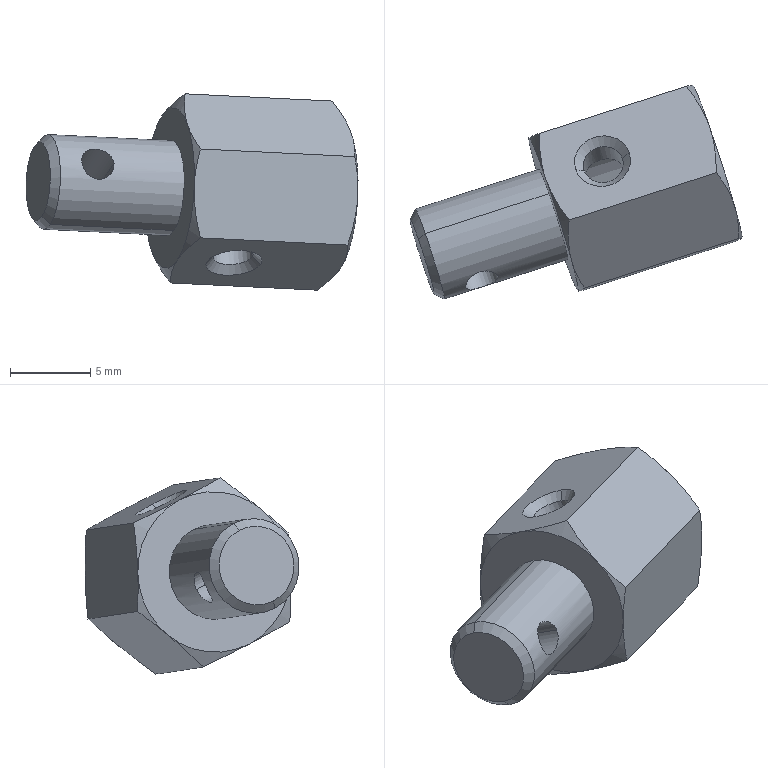Part | SolidWorks | features BaseBody 1 | 1 solid | 41 faces | box 20.658 x 13.325 x 12.212 mm | volume 845.345 mm3 | cone 22 | cylinder 10 | plane 9 | commonest cylinder face diameters 2.5 x4 2.1 x2 5.9 x2 6 x2
STEP:
#1=CARTESIAN_POINT('',(61.625,-75.237,-185.721));
#2=VERTEX_POINT('',#1);
#3=CARTESIAN_POINT('',(63.623,-74.596,-185.819));
#4=VERTEX_POINT('',#3);
#5=CARTESIAN_POINT('',(61.625,-75.237,-185.721));
#6=CARTESIAN_POINT('',(61.639,-75.298,-185.847));
#7=CARTESIAN_POINT('',(61.681,-75.358,-185.966));
#8=CARTESIAN_POINT('',(61.817,-75.465,-186.183));
#9=CARTESIAN_POINT('',(61.908,-75.512,-186.279));
#10=CARTESIAN_POINT('',(62.125,-75.58,-186.439));
#11=CARTESIAN_POINT('',(62.25,-75.6,-186.502));
#12=CARTESIAN_POINT('',(62.511,-75.599,-186.592));
#13=CARTESIAN_POINT('',(62.649,-75.578,-186.619));
#14=CARTESIAN_POINT('',(62.912,-75.494,-186.632));
#15=CARTESIAN_POINT('',(63.038,-75.43,-186.619));
#16=CARTESIAN_POINT('',(63.259,-75.275,-186.552));
#17=CARTESIAN_POINT('',(63.353,-75.186,-186.499));
#18=CARTESIAN_POINT('',(63.504,-75.,-186.357));
#19=CARTESIAN_POINT('',(63.559,-74.905,-186.268));
#20=CARTESIAN_POINT('',(63.625,-74.733,-186.061));
#21=CARTESIAN_POINT('',(63.636,-74.656,-185.943));
#22=CARTESIAN_POINT('',(63.623,-74.596,-185.819));
#23=B_SPLINE_CURVE_WITH_KNOTS('',3,(#5,#6,#7,#8,#9,#10,#11,#12,#13,#14,#15,#16,#17,#18,#19,#20,#21,#22),.UNSPECIFIED.,.F.,.F.,(4,2,2,2,2,2,2,2,4),(0.,0.000413,0.0008261,0.001239,0.001652,0.002065,0.002478,0.002891,0.003304),.UNSPECIFIED.);
#24=EDGE_CURVE('',#2,#4,#23,.T.);
#25=ORIENTED_EDGE('',*,*,#24,.T.);
#26=CARTESIAN_POINT('',(63.623,-74.596,-185.819));
#27=CARTESIAN_POINT('',(63.609,-74.536,-185.696));
#28=CARTESIAN_POINT('',(63.572,-74.493,-185.565));
#29=CARTESIAN_POINT('',(63.459,-74.445,-185.318));
#30=CARTESIAN_POINT('',(63.381,-74.439,-185.2));
#31=CARTESIAN_POINT('',(63.194,-74.457,-184.996));
#32=CARTESIAN_POINT('',(63.085,-74.48,-184.91));
#33=CARTESIAN_POINT('',(62.842,-74.543,-184.786));
#34=CARTESIAN_POINT('',(62.711,-74.583,-184.75));
#35=CARTESIAN_POINT('',(62.448,-74.667,-184.738));
#36=CARTESIAN_POINT('',(62.316,-74.713,-184.761));
#37=CARTESIAN_POINT('',(62.075,-74.804,-184.86));
#38=CARTESIAN_POINT('',(61.965,-74.852,-184.936));
#39=CARTESIAN_POINT('',(61.786,-74.952,-185.121));
#40=CARTESIAN_POINT('',(61.715,-75.005,-185.232));
#41=CARTESIAN_POINT('',(61.628,-75.117,-185.47));
#42=CARTESIAN_POINT('',(61.612,-75.177,-185.596));
#43=CARTESIAN_POINT('',(61.625,-75.237,-185.721));
#44=B_SPLINE_CURVE_WITH_KNOTS('',3,(#26,#27,#28,#29,#30,#31,#32,#33,#34,#35,#36,#37,#38,#39,#40,#41,#42,#43),.UNSPECIFIED.,.F.,.F.,(4,2,2,2,2,2,2,2,4),(0.003304,0.003717,0.004131,0.004544,0.004957,0.00537,0.005783,0.006196,0.006609),.UNSPECIFIED.);
#45=EDGE_CURVE('',#4,#2,#44,.T.);
#46=ORIENTED_EDGE('',*,*,#45,.T.);
#47=EDGE_LOOP('',(#25,#46));
#48=FACE_BOUND('',#47,.T.);
#49=CARTESIAN_POINT('',(61.395,-79.461,-186.994));
#50=VERTEX_POINT('',#49);
#51=CARTESIAN_POINT('',(60.832,-76.901,-181.708));
#52=VERTEX_POINT('',#51);
#53=CARTESIAN_POINT('',(61.113,-78.181,-184.351));
#54=DIRECTION('',(0.9511,0.3055,-0.04654));
#55=DIRECTION('',(-0.09549,0.4338,0.8959));
#56=AXIS2_PLACEMENT_3D('',#53,#54,#55);
#57=CIRCLE('',#56,2.95);
#58=EDGE_CURVE('',#50,#52,#57,.T.);
#59=ORIENTED_EDGE('',*,*,#58,.T.);
#60=CARTESIAN_POINT('',(68.535,-74.427,-182.085));
#61=VERTEX_POINT('',#60);
#62=CARTESIAN_POINT('',(60.356,-77.054,-181.684));
#63=DIRECTION('',(0.9511,0.3055,-0.04654));
#64=VECTOR('',#63,1000.);
#65=LINE('',#62,#64);
#66=EDGE_CURVE('',#52,#61,#65,.T.);
#67=ORIENTED_EDGE('',*,*,#66,.T.);
#68=CARTESIAN_POINT('',(69.099,-76.986,-187.371));
#69=VERTEX_POINT('',#68);
#70=CARTESIAN_POINT('',(68.817,-75.707,-184.728));
#71=DIRECTION('',(-0.9511,-0.3055,0.04654));
#72=DIRECTION('',(0.09549,-0.4338,-0.8959));
#73=AXIS2_PLACEMENT_3D('',#70,#71,#72);
#74=CIRCLE('',#73,2.95);
#75=EDGE_CURVE('',#61,#69,#74,.T.);
#76=ORIENTED_EDGE('',*,*,#75,.T.);
#77=CARTESIAN_POINT('',(60.919,-79.613,-186.971));
#78=DIRECTION('',(0.9511,0.3055,-0.04654));
#79=VECTOR('',#78,1000.);
#80=LINE('',#77,#79);
#81=EDGE_CURVE('',#50,#69,#80,.T.);
#82=ORIENTED_EDGE('',*,*,#81,.F.);
#83=EDGE_LOOP('',(#59,#67,#76,#82));
#84=FACE_OUTER_BOUND('',#83,.T.);
#85=CARTESIAN_POINT('',(60.638,-78.334,-184.328));
#86=DIRECTION('',(0.9511,0.3055,-0.04654));
#87=DIRECTION('',(0.09549,-0.4338,-0.8959));
#88=AXIS2_PLACEMENT_3D('',#85,#86,#87);
#89=CYLINDRICAL_SURFACE('',#88,2.95);
#90=ADVANCED_FACE('',(#48,#84),#89,.T.);
#91=CARTESIAN_POINT('',(60.404,-77.271,-182.132));
#92=VERTEX_POINT('',#91);
#93=CARTESIAN_POINT('',(60.872,-79.396,-186.523));
#94=VERTEX_POINT('',#93);
#95=CARTESIAN_POINT('',(60.638,-78.334,-184.328));
#96=DIRECTION('',(-0.9511,-0.3055,0.04654));
#97=DIRECTION('',(-0.09549,0.4338,0.8959));
#98=AXIS2_PLACEMENT_3D('',#95,#96,#97);
#99=CIRCLE('',#98,2.45);
#100=EDGE_CURVE('',#92,#94,#99,.T.);
#101=ORIENTED_EDGE('',*,*,#100,.F.);
#102=CARTESIAN_POINT('',(60.404,-77.271,-182.132));
#103=DIRECTION('',(0.605,0.5227,0.6006));
#104=VECTOR('',#103,1000.);
#105=LINE('',#102,#104);
#106=EDGE_CURVE('',#92,#52,#105,.T.);
#107=ORIENTED_EDGE('',*,*,#106,.T.);
#108=ORIENTED_EDGE('',*,*,#58,.F.);
#109=CARTESIAN_POINT('',(60.872,-79.396,-186.523));
#110=DIRECTION('',(0.74,-0.09071,-0.6664));
#111=VECTOR('',#110,1000.);
#112=LINE('',#109,#111);
#113=EDGE_CURVE('',#94,#50,#112,.T.);
#114=ORIENTED_EDGE('',*,*,#113,.F.);
#115=EDGE_LOOP('',(#101,#107,#108,#114));
#116=FACE_OUTER_BOUND('',#115,.T.);
#117=CARTESIAN_POINT('',(60.638,-78.334,-184.328));
#118=DIRECTION('',(0.9511,0.3055,-0.04654));
#119=DIRECTION('',(0.09549,-0.4338,-0.8959));
#120=AXIS2_PLACEMENT_3D('',#117,#118,#119);
#121=CONICAL_SURFACE('',#120,2.45,0.7854);
#122=ADVANCED_FACE('',(#116),#121,.T.);
#123=CARTESIAN_POINT('',(70.147,-73.886,-182.119));
#124=VERTEX_POINT('',#123);
#125=CARTESIAN_POINT('',(70.72,-76.488,-187.495));
#126=VERTEX_POINT('',#125);
#127=CARTESIAN_POINT('',(70.434,-75.187,-184.807));
#128=DIRECTION('',(0.9511,0.3055,-0.04654));
#129=DIRECTION('',(0.09549,-0.4338,-0.8959));
#130=AXIS2_PLACEMENT_3D('',#127,#128,#129);
#131=CIRCLE('',#130,3.);
#132=EDGE_CURVE('',#124,#126,#131,.T.);
#133=ORIENTED_EDGE('',*,*,#132,.F.);
#134=CARTESIAN_POINT('',(70.86,-73.657,-182.154));
#135=VERTEX_POINT('',#134);
#136=CARTESIAN_POINT('',(70.147,-73.886,-182.119));
#137=DIRECTION('',(0.9511,0.3055,-0.04654));
#138=VECTOR('',#137,1000.);
#139=LINE('',#136,#138);
#140=EDGE_CURVE('',#124,#135,#139,.T.);
#141=ORIENTED_EDGE('',*,*,#140,.T.);
#142=CARTESIAN_POINT('',(73.238,-72.893,-182.27));
#143=VERTEX_POINT('',#142);
#144=CARTESIAN_POINT('',(70.86,-73.657,-182.154));
#145=CARTESIAN_POINT('',(70.909,-73.796,-182.081));
#146=CARTESIAN_POINT('',(70.991,-73.933,-182.022));
#147=CARTESIAN_POINT('',(71.204,-74.172,-181.939));
#148=CARTESIAN_POINT('',(71.335,-74.275,-181.913));
#149=CARTESIAN_POINT('',(71.555,-74.391,-181.893));
#150=CARTESIAN_POINT('',(71.631,-74.423,-181.889));
#151=CARTESIAN_POINT('',(71.788,-74.473,-181.885));
#152=CARTESIAN_POINT('',(71.871,-74.491,-181.885));
#153=CARTESIAN_POINT('',(72.035,-74.509,-181.888));
#154=CARTESIAN_POINT('',(72.117,-74.51,-181.891));
#155=CARTESIAN_POINT('',(72.281,-74.495,-181.897));
#156=CARTESIAN_POINT('',(72.364,-74.478,-181.901));
#157=CARTESIAN_POINT('',(72.599,-74.403,-181.912));
#158=CARTESIAN_POINT('',(72.746,-74.317,-181.92));
#159=CARTESIAN_POINT('',(72.99,-74.095,-181.943));
#160=CARTESIAN_POINT('',(73.09,-73.96,-181.958));
#161=CARTESIAN_POINT('',(73.234,-73.665,-182.006));
#162=CARTESIAN_POINT('',(73.278,-73.507,-182.04));
#163=CARTESIAN_POINT('',(73.305,-73.189,-182.136));
#164=CARTESIAN_POINT('',(73.287,-73.035,-182.196));
#165=CARTESIAN_POINT('',(73.238,-72.893,-182.27));
#166=B_SPLINE_CURVE_WITH_KNOTS('',3,(#144,#145,#146,#147,#148,#149,#150,#151,#152,#153,#154,#155,#156,#157,#158,#159,#160,#161,#162,#163,#164,#165),.UNSPECIFIED.,.F.,.F.,(4,2,2,2,2,2,2,2,2,2,4),(0.003954,0.004448,0.004941,0.005188,0.005435,0.005682,0.005929,0.006423,0.006917,0.00741,0.007904),.UNSPECIFIED.);
#167=EDGE_CURVE('',#135,#143,#166,.T.);
#168=ORIENTED_EDGE('',*,*,#167,.T.);
#169=CARTESIAN_POINT('',(78.231,-71.289,-182.515));
#170=VERTEX_POINT('',#169);
#171=CARTESIAN_POINT('',(70.147,-73.886,-182.119));
#172=DIRECTION('',(0.9511,0.3055,-0.04654));
#173=VECTOR('',#172,1000.);
#174=LINE('',#171,#173);
#175=EDGE_CURVE('',#143,#170,#174,.T.);
#176=ORIENTED_EDGE('',*,*,#175,.T.);
#177=CARTESIAN_POINT('',(78.804,-73.892,-187.89));
#178=VERTEX_POINT('',#177);
#179=CARTESIAN_POINT('',(78.518,-72.59,-185.202));
#180=DIRECTION('',(0.9511,0.3055,-0.04654));
#181=DIRECTION('',(0.09549,-0.4338,-0.8959));
#182=AXIS2_PLACEMENT_3D('',#179,#180,#181);
#183=CIRCLE('',#182,3.);
#184=EDGE_CURVE('',#170,#178,#183,.T.);
#185=ORIENTED_EDGE('',*,*,#184,.T.);
#186=CARTESIAN_POINT('',(73.811,-75.496,-187.646));
#187=VERTEX_POINT('',#186);
#188=CARTESIAN_POINT('',(70.72,-76.488,-187.495));
#189=DIRECTION('',(0.9511,0.3055,-0.04654));
#190=VECTOR('',#189,1000.);
#191=LINE('',#188,#190);
#192=EDGE_CURVE('',#187,#178,#191,.T.);
#193=ORIENTED_EDGE('',*,*,#192,.F.);
#194=CARTESIAN_POINT('',(71.433,-76.259,-187.53));
#195=VERTEX_POINT('',#194);
#196=CARTESIAN_POINT('',(73.811,-75.496,-187.646));
#197=CARTESIAN_POINT('',(73.859,-75.635,-187.573));
#198=CARTESIAN_POINT('',(73.875,-75.78,-187.486));
#199=CARTESIAN_POINT('',(73.839,-76.054,-187.302));
#200=CARTESIAN_POINT('',(73.788,-76.183,-187.206));
#201=CARTESIAN_POINT('',(73.67,-76.358,-187.075));
#202=CARTESIAN_POINT('',(73.624,-76.413,-187.033));
#203=CARTESIAN_POINT('',(73.52,-76.516,-186.958));
#204=CARTESIAN_POINT('',(73.46,-76.564,-186.923));
#205=CARTESIAN_POINT('',(73.333,-76.652,-186.865));
#206=CARTESIAN_POINT('',(73.265,-76.692,-186.841));
#207=CARTESIAN_POINT('',(73.12,-76.762,-186.806));
#208=CARTESIAN_POINT('',(73.042,-76.793,-186.795));
#209=CARTESIAN_POINT('',(72.807,-76.869,-186.784));
#210=CARTESIAN_POINT('',(72.641,-76.898,-186.805));
#211=CARTESIAN_POINT('',(72.323,-76.906,-186.893));
#212=CARTESIAN_POINT('',(72.169,-76.886,-186.96));
#213=CARTESIAN_POINT('',(71.89,-76.792,-187.114));
#214=CARTESIAN_POINT('',(71.766,-76.72,-187.2));
#215=CARTESIAN_POINT('',(71.56,-76.523,-187.373));
#216=CARTESIAN_POINT('',(71.482,-76.401,-187.456));
#217=CARTESIAN_POINT('',(71.433,-76.259,-187.53));
#218=B_SPLINE_CURVE_WITH_KNOTS('',3,(#196,#197,#198,#199,#200,#201,#202,#203,#204,#205,#206,#207,#208,#209,#210,#211,#212,#213,#214,#215,#216,#217),.UNSPECIFIED.,.F.,.F.,(4,2,2,2,2,2,2,2,2,2,4),(0.003954,0.004448,0.004941,0.005188,0.005435,0.005682,0.005929,0.006423,0.006917,0.00741,0.007904),.UNSPECIFIED.);
#219=EDGE_CURVE('',#187,#195,#218,.T.);
#220=ORIENTED_EDGE('',*,*,#219,.T.);
#221=CARTESIAN_POINT('',(70.72,-76.488,-187.495));
#222=DIRECTION('',(0.9511,0.3055,-0.04654));
#223=VECTOR('',#222,1000.);
#224=LINE('',#221,#223);
#225=EDGE_CURVE('',#126,#195,#224,.T.);
#226=ORIENTED_EDGE('',*,*,#225,.F.);
#227=EDGE_LOOP('',(#133,#141,#168,#176,#185,#193,#220,#226));
#228=FACE_OUTER_BOUND('',#227,.T.);
#229=CARTESIAN_POINT('',(70.434,-75.187,-184.807));
#230=DIRECTION('',(0.9511,0.3055,-0.04654));
#231=DIRECTION('',(0.09549,-0.4338,-0.8959));
#232=AXIS2_PLACEMENT_3D('',#229,#230,#231);
#233=CYLINDRICAL_SURFACE('',#232,3.);
#234=ADVANCED_FACE('',(#228),#233,.F.);
#235=CARTESIAN_POINT('',(68.786,-75.716,-184.726));
#236=VERTEX_POINT('',#235);
#237=CARTESIAN_POINT('',(70.72,-76.488,-187.495));
#238=DIRECTION('',(0.5582,-0.2229,-0.7992));
#239=VECTOR('',#238,1000.);
#240=LINE('',#237,#239);
#241=EDGE_CURVE('',#236,#126,#240,.T.);
#242=ORIENTED_EDGE('',*,*,#241,.F.);
#243=CARTESIAN_POINT('',(70.147,-73.886,-182.119));
#244=DIRECTION('',(0.3928,0.5284,0.7526));
#245=VECTOR('',#244,1000.);
#246=LINE('',#243,#245);
#247=EDGE_CURVE('',#236,#124,#246,.T.);
#248=ORIENTED_EDGE('',*,*,#247,.T.);
#249=ORIENTED_EDGE('',*,*,#132,.T.);
#250=EDGE_LOOP('',(#242,#248,#249));
#251=FACE_OUTER_BOUND('',#250,.T.);
#252=CARTESIAN_POINT('',(70.434,-75.187,-184.807));
#253=DIRECTION('',(0.9511,0.3055,-0.04654));
#254=DIRECTION('',(0.09549,-0.4338,-0.8959));
#255=AXIS2_PLACEMENT_3D('',#252,#253,#254);
#256=CONICAL_SURFACE('',#255,3.,1.047);
#257=ADVANCED_FACE('',(#251),#256,.F.);
#258=ORIENTED_EDGE('',*,*,#184,.F.);
#259=CARTESIAN_POINT('',(78.659,-70.92,-182.09));
#260=VERTEX_POINT('',#259);
#261=CARTESIAN_POINT('',(78.231,-71.289,-182.515));
#262=DIRECTION('',(0.605,0.5227,0.6006));
#263=VECTOR('',#262,1000.);
#264=LINE('',#261,#263);
#265=EDGE_CURVE('',#170,#260,#264,.T.);
#266=ORIENTED_EDGE('',*,*,#265,.T.);
#267=CARTESIAN_POINT('',(79.327,-73.956,-188.362));
#268=VERTEX_POINT('',#267);
#269=CARTESIAN_POINT('',(78.993,-72.438,-185.226));
#270=DIRECTION('',(-0.9511,-0.3055,0.04654));
#271=DIRECTION('',(0.09549,-0.4338,-0.8959));
#272=AXIS2_PLACEMENT_3D('',#269,#270,#271);
#273=CIRCLE('',#272,3.5);
#274=EDGE_CURVE('',#268,#260,#273,.T.);
#275=ORIENTED_EDGE('',*,*,#274,.F.);
#276=CARTESIAN_POINT('',(78.804,-73.892,-187.89));
#277=DIRECTION('',(0.74,-0.09071,-0.6664));
#278=VECTOR('',#277,1000.);
#279=LINE('',#276,#278);
#280=EDGE_CURVE('',#178,#268,#279,.T.);
#281=ORIENTED_EDGE('',*,*,#280,.F.);
#282=EDGE_LOOP('',(#258,#266,#275,#281));
#283=FACE_OUTER_BOUND('',#282,.T.);
#284=CARTESIAN_POINT('',(78.518,-72.59,-185.202));
#285=DIRECTION('',(0.9511,0.3055,-0.04654));
#286=DIRECTION('',(0.09549,-0.4338,-0.8959));
#287=AXIS2_PLACEMENT_3D('',#284,#285,#286);
#288=CONICAL_SURFACE('',#287,3.,0.7854);
#289=ADVANCED_FACE('',(#283),#288,.F.);
#290=ORIENTED_EDGE('',*,*,#167,.F.);
#291=CARTESIAN_POINT('',(70.717,-73.006,-180.81));
#292=VERTEX_POINT('',#291);
#293=CARTESIAN_POINT('',(71.624,-77.127,-189.322));
#294=DIRECTION('',(-0.09549,0.4338,0.8959));
#295=VECTOR('',#294,1000.);
#296=LINE('',#293,#295);
#297=EDGE_CURVE('',#135,#292,#296,.T.);
#298=ORIENTED_EDGE('',*,*,#297,.T.);
#299=CARTESIAN_POINT('',(73.095,-72.242,-180.926));
#300=VERTEX_POINT('',#299);
#301=CARTESIAN_POINT('',(71.906,-72.624,-180.868));
#302=DIRECTION('',(-0.09549,0.4338,0.8959));
#303=DIRECTION('',(-0.9511,-0.3055,0.04654));
#304=AXIS2_PLACEMENT_3D('',#301,#302,#303);
#305=CIRCLE('',#304,1.25);
#306=EDGE_CURVE('',#292,#300,#305,.T.);
#307=ORIENTED_EDGE('',*,*,#306,.T.);
#308=CARTESIAN_POINT('',(74.002,-76.363,-189.438));
#309=DIRECTION('',(-0.09549,0.4338,0.8959));
#310=VECTOR('',#309,1000.);
#311=LINE('',#308,#310);
#312=EDGE_CURVE('',#143,#300,#311,.T.);
#313=ORIENTED_EDGE('',*,*,#312,.F.);
#314=EDGE_LOOP('',(#290,#298,#307,#313));
#315=FACE_OUTER_BOUND('',#314,.T.);
#316=CARTESIAN_POINT('',(72.813,-76.745,-189.38));
#317=DIRECTION('',(-0.09549,0.4338,0.8959));
#318=DIRECTION('',(0.9511,0.3055,-0.04654));
#319=AXIS2_PLACEMENT_3D('',#316,#317,#318);
#320=CYLINDRICAL_SURFACE('',#319,1.25);
#321=ADVANCED_FACE('',(#315),#320,.F.);
#322=CARTESIAN_POINT('',(73.954,-76.146,-188.99));
#323=VERTEX_POINT('',#322);
#324=CARTESIAN_POINT('',(71.577,-76.91,-188.874));
#325=VERTEX_POINT('',#324);
#326=CARTESIAN_POINT('',(72.765,-76.528,-188.932));
#327=DIRECTION('',(0.09549,-0.4338,-0.8959));
#328=DIRECTION('',(0.9511,0.3055,-0.04654));
#329=AXIS2_PLACEMENT_3D('',#326,#327,#328);
#330=CIRCLE('',#329,1.25);
#331=EDGE_CURVE('',#323,#325,#330,.T.);
#332=ORIENTED_EDGE('',*,*,#331,.T.);
#333=CARTESIAN_POINT('',(71.624,-77.127,-189.322));
#334=DIRECTION('',(-0.09549,0.4338,0.8959));
#335=VECTOR('',#334,1000.);
#336=LINE('',#333,#335);
#337=EDGE_CURVE('',#325,#195,#336,.T.);
#338=ORIENTED_EDGE('',*,*,#337,.T.);
#339=ORIENTED_EDGE('',*,*,#219,.F.);
#340=CARTESIAN_POINT('',(74.002,-76.363,-189.438));
#341=DIRECTION('',(-0.09549,0.4338,0.8959));
#342=VECTOR('',#341,1000.);
#343=LINE('',#340,#342);
#344=EDGE_CURVE('',#323,#187,#343,.T.);
#345=ORIENTED_EDGE('',*,*,#344,.F.);
#346=EDGE_LOOP('',(#332,#338,#339,#345));
#347=FACE_OUTER_BOUND('',#346,.T.);
#348=CARTESIAN_POINT('',(72.813,-76.745,-189.38));
#349=DIRECTION('',(-0.09549,0.4338,0.8959));
#350=DIRECTION('',(0.9511,0.3055,-0.04654));
#351=AXIS2_PLACEMENT_3D('',#348,#349,#350);
#352=CYLINDRICAL_SURFACE('',#351,1.25);
#353=ADVANCED_FACE('',(#347),#352,.F.);
#354=ORIENTED_EDGE('',*,*,#306,.F.);
#355=CARTESIAN_POINT('',(70.194,-72.942,-180.339));
#356=VERTEX_POINT('',#355);
#357=CARTESIAN_POINT('',(70.717,-73.006,-180.81));
#358=DIRECTION('',(-0.74,0.09071,0.6664));
#359=VECTOR('',#358,1000.);
#360=LINE('',#357,#359);
#361=EDGE_CURVE('',#292,#356,#360,.T.);
#362=ORIENTED_EDGE('',*,*,#361,.T.);
#363=CARTESIAN_POINT('',(73.523,-71.873,-180.502));
#364=VERTEX_POINT('',#363);
#365=CARTESIAN_POINT('',(71.858,-72.407,-180.42));
#366=DIRECTION('',(0.09549,-0.4338,-0.8959));
#367=DIRECTION('',(-0.9511,-0.3055,0.04654));
#368=AXIS2_PLACEMENT_3D('',#365,#366,#367);
#369=CIRCLE('',#368,1.75);
#370=EDGE_CURVE('',#364,#356,#369,.T.);
#371=ORIENTED_EDGE('',*,*,#370,.F.);
#372=CARTESIAN_POINT('',(73.095,-72.242,-180.926));
#373=DIRECTION('',(0.605,0.5227,0.6006));
#374=VECTOR('',#373,1000.);
#375=LINE('',#372,#374);
#376=EDGE_CURVE('',#300,#364,#375,.T.);
#377=ORIENTED_EDGE('',*,*,#376,.F.);
#378=EDGE_LOOP('',(#354,#362,#371,#377));
#379=FACE_OUTER_BOUND('',#378,.T.);
#380=CARTESIAN_POINT('',(71.906,-72.624,-180.868));
#381=DIRECTION('',(-0.09549,0.4338,0.8959));
#382=DIRECTION('',(0.9511,0.3055,-0.04654));
#383=AXIS2_PLACEMENT_3D('',#380,#381,#382);
#384=CONICAL_SURFACE('',#383,1.25,0.7854);
#385=ADVANCED_FACE('',(#379),#384,.F.);
#386=ORIENTED_EDGE('',*,*,#331,.F.);
#387=CARTESIAN_POINT('',(74.478,-76.21,-189.461));
#388=VERTEX_POINT('',#387);
#389=CARTESIAN_POINT('',(74.478,-76.21,-189.461));
#390=DIRECTION('',(0.74,-0.09071,-0.6664));
#391=VECTOR('',#390,1000.);
#392=LINE('',#389,#391);
#393=EDGE_CURVE('',#323,#388,#392,.T.);
#394=ORIENTED_EDGE('',*,*,#393,.T.);
#395=CARTESIAN_POINT('',(71.149,-77.28,-189.298));
#396=VERTEX_POINT('',#395);
#397=CARTESIAN_POINT('',(72.813,-76.745,-189.38));
#398=DIRECTION('',(-0.09549,0.4338,0.8959));
#399=DIRECTION('',(0.9511,0.3055,-0.04654));
#400=AXIS2_PLACEMENT_3D('',#397,#398,#399);
#401=CIRCLE('',#400,1.75);
#402=EDGE_CURVE('',#396,#388,#401,.T.);
#403=ORIENTED_EDGE('',*,*,#402,.F.);
#404=CARTESIAN_POINT('',(71.149,-77.28,-189.298));
#405=DIRECTION('',(-0.605,-0.5227,-0.6006));
#406=VECTOR('',#405,1000.);
#407=LINE('',#404,#406);
#408=EDGE_CURVE('',#325,#396,#407,.T.);
#409=ORIENTED_EDGE('',*,*,#408,.F.);
#410=EDGE_LOOP('',(#386,#394,#403,#409));
#411=FACE_OUTER_BOUND('',#410,.T.);
#412=CARTESIAN_POINT('',(72.813,-76.745,-189.38));
#413=DIRECTION('',(0.09549,-0.4338,-0.8959));
#414=DIRECTION('',(-0.9511,-0.3055,0.04654));
#415=AXIS2_PLACEMENT_3D('',#412,#413,#414);
#416=CONICAL_SURFACE('',#415,1.75,0.7854);
#417=ADVANCED_FACE('',(#411),#416,.F.);
#418=CARTESIAN_POINT('',(65.356,-79.597,-183.213));
#419=VERTEX_POINT('',#418);
#420=CARTESIAN_POINT('',(63.359,-80.239,-183.115));
#421=VERTEX_POINT('',#420);
#422=CARTESIAN_POINT('',(65.356,-79.597,-183.213));
#423=CARTESIAN_POINT('',(65.37,-79.657,-183.336));
#424=CARTESIAN_POINT('',(65.353,-79.717,-183.464));
#425=CARTESIAN_POINT('',(65.267,-79.829,-183.701));
#426=CARTESIAN_POINT('',(65.197,-79.882,-183.812));
#427=CARTESIAN_POINT('',(65.017,-79.982,-183.999));
#428=CARTESIAN_POINT('',(64.908,-80.03,-184.074));
#429=CARTESIAN_POINT('',(64.664,-80.123,-184.174));
#430=CARTESIAN_POINT('',(64.532,-80.167,-184.197));
#431=CARTESIAN_POINT('',(64.269,-80.252,-184.184));
#432=CARTESIAN_POINT('',(64.138,-80.292,-184.147));
#433=CARTESIAN_POINT('',(63.899,-80.354,-184.025));
#434=CARTESIAN_POINT('',(63.788,-80.377,-183.939));
#435=CARTESIAN_POINT('',(63.602,-80.395,-183.736));
#436=CARTESIAN_POINT('',(63.524,-80.39,-183.617));
#437=CARTESIAN_POINT('',(63.409,-80.342,-183.369));
#438=CARTESIAN_POINT('',(63.373,-80.299,-183.241));
#439=CARTESIAN_POINT('',(63.359,-80.239,-183.115));
#440=B_SPLINE_CURVE_WITH_KNOTS('',3,(#422,#423,#424,#425,#426,#427,#428,#429,#430,#431,#432,#433,#434,#435,#436,#437,#438,#439),.UNSPECIFIED.,.F.,.F.,(4,2,2,2,2,2,2,2,4),(0.003304,0.003717,0.004131,0.004544,0.004957,0.00537,0.005783,0.006196,0.006609),.UNSPECIFIED.);
#441=EDGE_CURVE('',#419,#421,#440,.T.);
#442=ORIENTED_EDGE('',*,*,#441,.F.);
#443=CARTESIAN_POINT('',(66.106,-81.759,-182.087));
#444=DIRECTION('',(-0.2939,0.8477,-0.4417));
#445=VECTOR('',#444,1000.);
#446=LINE('',#443,#445);
#447=EDGE_CURVE('',#419,#4,#446,.T.);
#448=ORIENTED_EDGE('',*,*,#447,.T.);
#449=ORIENTED_EDGE('',*,*,#24,.F.);
#450=CARTESIAN_POINT('',(64.109,-82.4,-181.989));
#451=DIRECTION('',(-0.2939,0.8477,-0.4417));
#452=VECTOR('',#451,1000.);
#453=LINE('',#450,#452);
#454=EDGE_CURVE('',#421,#2,#453,.T.);
#455=ORIENTED_EDGE('',*,*,#454,.F.);
#456=EDGE_LOOP('',(#442,#448,#449,#455));
#457=FACE_OUTER_BOUND('',#456,.T.);
#458=CARTESIAN_POINT('',(65.107,-82.079,-182.038));
#459=DIRECTION('',(-0.2939,0.8477,-0.4417));
#460=DIRECTION('',(-0.9511,-0.3055,0.04654));
#461=AXIS2_PLACEMENT_3D('',#458,#459,#460);
#462=CYLINDRICAL_SURFACE('',#461,1.05);
#463=ADVANCED_FACE('',(#457),#462,.F.);
#464=ORIENTED_EDGE('',*,*,#447,.F.);
#465=CARTESIAN_POINT('',(63.359,-80.239,-183.115));
#466=CARTESIAN_POINT('',(63.346,-80.178,-182.99));
#467=CARTESIAN_POINT('',(63.356,-80.102,-182.873));
#468=CARTESIAN_POINT('',(63.422,-79.929,-182.666));
#469=CARTESIAN_POINT('',(63.478,-79.835,-182.577));
#470=CARTESIAN_POINT('',(63.628,-79.65,-182.436));
#471=CARTESIAN_POINT('',(63.723,-79.559,-182.382));
#472=CARTESIAN_POINT('',(63.943,-79.405,-182.316));
#473=CARTESIAN_POINT('',(64.069,-79.341,-182.302));
#474=CARTESIAN_POINT('',(64.332,-79.256,-182.315));
#475=CARTESIAN_POINT('',(64.469,-79.236,-182.341));
#476=CARTESIAN_POINT('',(64.732,-79.235,-182.432));
#477=CARTESIAN_POINT('',(64.856,-79.255,-182.495));
#478=CARTESIAN_POINT('',(65.074,-79.322,-182.655));
#479=CARTESIAN_POINT('',(65.165,-79.369,-182.751));
#480=CARTESIAN_POINT('',(65.3,-79.477,-182.968));
#481=CARTESIAN_POINT('',(65.343,-79.537,-183.089));
#482=CARTESIAN_POINT('',(65.356,-79.597,-183.213));
#483=B_SPLINE_CURVE_WITH_KNOTS('',3,(#465,#466,#467,#468,#469,#470,#471,#472,#473,#474,#475,#476,#477,#478,#479,#480,#481,#482),.UNSPECIFIED.,.F.,.F.,(4,2,2,2,2,2,2,2,4),(0.,0.000413,0.0008261,0.001239,0.001652,0.002065,0.002478,0.002891,0.003304),.UNSPECIFIED.);
#484=EDGE_CURVE('',#421,#419,#483,.T.);
#485=ORIENTED_EDGE('',*,*,#484,.F.);
#486=ORIENTED_EDGE('',*,*,#454,.T.);
#487=ORIENTED_EDGE('',*,*,#45,.F.);
#488=EDGE_LOOP('',(#464,#485,#486,#487));
#489=FACE_OUTER_BOUND('',#488,.T.);
#490=CARTESIAN_POINT('',(65.107,-82.079,-182.038));
#491=DIRECTION('',(-0.2939,0.8477,-0.4417));
#492=DIRECTION('',(-0.9511,-0.3055,0.04654));
#493=AXIS2_PLACEMENT_3D('',#490,#491,#492);
#494=CYLINDRICAL_SURFACE('',#493,1.05);
#495=ADVANCED_FACE('',(#489),#494,.F.);
#496=ORIENTED_EDGE('',*,*,#393,.F.);
#497=CARTESIAN_POINT('',(72.765,-76.528,-188.932));
#498=DIRECTION('',(0.09549,-0.4338,-0.8959));
#499=DIRECTION('',(0.9511,0.3055,-0.04654));
#500=AXIS2_PLACEMENT_3D('',#497,#498,#499);
#501=CIRCLE('',#500,1.25);
#502=EDGE_CURVE('',#325,#323,#501,.T.);
#503=ORIENTED_EDGE('',*,*,#502,.F.);
#504=ORIENTED_EDGE('',*,*,#408,.T.);
#505=CARTESIAN_POINT('',(72.813,-76.745,-189.38));
#506=DIRECTION('',(-0.09549,0.4338,0.8959));
#507=DIRECTION('',(0.9511,0.3055,-0.04654));
#508=AXIS2_PLACEMENT_3D('',#505,#506,#507);
#509=CIRCLE('',#508,1.75);
#510=EDGE_CURVE('',#388,#396,#509,.T.);
#511=ORIENTED_EDGE('',*,*,#510,.F.);
#512=EDGE_LOOP('',(#496,#503,#504,#511));
#513=FACE_OUTER_BOUND('',#512,.T.);
#514=CARTESIAN_POINT('',(72.813,-76.745,-189.38));
#515=DIRECTION('',(0.09549,-0.4338,-0.8959));
#516=DIRECTION('',(-0.9511,-0.3055,0.04654));
#517=AXIS2_PLACEMENT_3D('',#514,#515,#516);
#518=CONICAL_SURFACE('',#517,1.75,0.7854);
#519=ADVANCED_FACE('',(#513),#518,.F.);
#520=ORIENTED_EDGE('',*,*,#361,.F.);
#521=CARTESIAN_POINT('',(71.906,-72.624,-180.868));
#522=DIRECTION('',(-0.09549,0.4338,0.8959));
#523=DIRECTION('',(-0.9511,-0.3055,0.04654));
#524=AXIS2_PLACEMENT_3D('',#521,#522,#523);
#525=CIRCLE('',#524,1.25);
#526=EDGE_CURVE('',#300,#292,#525,.T.);
#527=ORIENTED_EDGE('',*,*,#526,.F.);
#528=ORIENTED_EDGE('',*,*,#376,.T.);
#529=CARTESIAN_POINT('',(71.858,-72.407,-180.42));
#530=DIRECTION('',(0.09549,-0.4338,-0.8959));
#531=DIRECTION('',(-0.9511,-0.3055,0.04654));
#532=AXIS2_PLACEMENT_3D('',#529,#530,#531);
#533=CIRCLE('',#532,1.75);
#534=EDGE_CURVE('',#356,#364,#533,.T.);
#535=ORIENTED_EDGE('',*,*,#534,.F.);
#536=EDGE_LOOP('',(#520,#527,#528,#535));
#537=FACE_OUTER_BOUND('',#536,.T.);
#538=CARTESIAN_POINT('',(71.906,-72.624,-180.868));
#539=DIRECTION('',(-0.09549,0.4338,0.8959));
#540=DIRECTION('',(0.9511,0.3055,-0.04654));
#541=AXIS2_PLACEMENT_3D('',#538,#539,#540);
#542=CONICAL_SURFACE('',#541,1.25,0.7854);
#543=ADVANCED_FACE('',(#537),#542,.F.);
#544=ORIENTED_EDGE('',*,*,#337,.F.);
#545=ORIENTED_EDGE('',*,*,#502,.T.);
#546=ORIENTED_EDGE('',*,*,#344,.T.);
#547=CARTESIAN_POINT('',(71.433,-76.259,-187.53));
#548=CARTESIAN_POINT('',(71.409,-76.188,-187.567));
#549=CARTESIAN_POINT('',(71.392,-76.115,-187.6));
#550=CARTESIAN_POINT('',(71.374,-75.963,-187.661));
#551=CARTESIAN_POINT('',(71.373,-75.883,-187.688));
#552=CARTESIAN_POINT('',(71.393,-75.646,-187.76));
#553=CARTESIAN_POINT('',(71.438,-75.486,-187.794));
#554=CARTESIAN_POINT('',(71.581,-75.193,-187.842));
#555=CARTESIAN_POINT('',(71.681,-75.057,-187.857));
#556=CARTESIAN_POINT('',(71.925,-74.837,-187.88));
#557=CARTESIAN_POINT('',(72.071,-74.75,-187.888));
#558=CARTESIAN_POINT('',(72.307,-74.675,-187.899));
#559=CARTESIAN_POINT('',(72.389,-74.658,-187.903));
#560=CARTESIAN_POINT('',(72.553,-74.642,-187.909));
#561=CARTESIAN_POINT('',(72.636,-74.643,-187.912));
#562=CARTESIAN_POINT('',(72.885,-74.671,-187.916));
#563=CARTESIAN_POINT('',(73.045,-74.723,-187.914));
#564=CARTESIAN_POINT('',(73.336,-74.878,-187.886));
#565=CARTESIAN_POINT('',(73.468,-74.981,-187.861));
#566=CARTESIAN_POINT('',(73.68,-75.219,-187.778));
#567=CARTESIAN_POINT('',(73.763,-75.356,-187.719));
#568=CARTESIAN_POINT('',(73.811,-75.496,-187.646));
#569=B_SPLINE_CURVE_WITH_KNOTS('',3,(#547,#548,#549,#550,#551,#552,#553,#554,#555,#556,#557,#558,#559,#560,#561,#562,#563,#564,#565,#566,#567,#568),.UNSPECIFIED.,.F.,.F.,(4,2,2,2,2,2,2,2,2,2,4),(0.,0.0002471,0.0004942,0.0009884,0.001483,0.001977,0.002224,0.002471,0.002965,0.003459,0.003954),.UNSPECIFIED.);
#570=EDGE_CURVE('',#195,#187,#569,.T.);
#571=ORIENTED_EDGE('',*,*,#570,.F.);
#572=EDGE_LOOP('',(#544,#545,#546,#571));
#573=FACE_OUTER_BOUND('',#572,.T.);
#574=CARTESIAN_POINT('',(72.813,-76.745,-189.38));
#575=DIRECTION('',(-0.09549,0.4338,0.8959));
#576=DIRECTION('',(0.9511,0.3055,-0.04654));
#577=AXIS2_PLACEMENT_3D('',#574,#575,#576);
#578=CYLINDRICAL_SURFACE('',#577,1.25);
#579=ADVANCED_FACE('',(#573),#578,.F.);
#580=ORIENTED_EDGE('',*,*,#297,.F.);
#581=CARTESIAN_POINT('',(73.238,-72.893,-182.27));
#582=CARTESIAN_POINT('',(73.213,-72.822,-182.307));
#583=CARTESIAN_POINT('',(73.182,-72.757,-182.346));
#584=CARTESIAN_POINT('',(73.105,-72.636,-182.428));
#585=CARTESIAN_POINT('',(73.059,-72.58,-182.471));
#586=CARTESIAN_POINT('',(72.906,-72.433,-182.6));
#587=CARTESIAN_POINT('',(72.781,-72.36,-182.687));
#588=CARTESIAN_POINT('',(72.504,-72.267,-182.84));
#589=CARTESIAN_POINT('',(72.349,-72.246,-182.907));
#590=CARTESIAN_POINT('',(72.032,-72.254,-182.995));
#591=CARTESIAN_POINT('',(71.866,-72.283,-183.016));
#592=CARTESIAN_POINT('',(71.63,-72.359,-183.005));
#593=CARTESIAN_POINT('',(71.552,-72.39,-182.994));
#594=CARTESIAN_POINT('',(71.407,-72.46,-182.959));
#595=CARTESIAN_POINT('',(71.339,-72.5,-182.935));
#596=CARTESIAN_POINT('',(71.146,-72.633,-182.847));
#597=CARTESIAN_POINT('',(71.04,-72.737,-182.768));
#598=CARTESIAN_POINT('',(70.883,-72.97,-182.593));
#599=CARTESIAN_POINT('',(70.832,-73.1,-182.497));
#600=CARTESIAN_POINT('',(70.797,-73.372,-182.315));
#601=CARTESIAN_POINT('',(70.812,-73.517,-182.227));
#602=CARTESIAN_POINT('',(70.86,-73.657,-182.154));
#603=B_SPLINE_CURVE_WITH_KNOTS('',3,(#581,#582,#583,#584,#585,#586,#587,#588,#589,#590,#591,#592,#593,#594,#595,#596,#597,#598,#599,#600,#601,#602),.UNSPECIFIED.,.F.,.F.,(4,2,2,2,2,2,2,2,2,2,4),(0.,0.0002471,0.0004942,0.0009884,0.001483,0.001977,0.002224,0.002471,0.002965,0.003459,0.003954),.UNSPECIFIED.);
#604=EDGE_CURVE('',#143,#135,#603,.T.);
#605=ORIENTED_EDGE('',*,*,#604,.F.);
#606=ORIENTED_EDGE('',*,*,#312,.T.);
#607=ORIENTED_EDGE('',*,*,#526,.T.);
#608=EDGE_LOOP('',(#580,#605,#606,#607));
#609=FACE_OUTER_BOUND('',#608,.T.);
#610=CARTESIAN_POINT('',(72.813,-76.745,-189.38));
#611=DIRECTION('',(-0.09549,0.4338,0.8959));
#612=DIRECTION('',(0.9511,0.3055,-0.04654));
#613=AXIS2_PLACEMENT_3D('',#610,#611,#612);
#614=CYLINDRICAL_SURFACE('',#613,1.25);
#615=ADVANCED_FACE('',(#609),#614,.F.);
#616=ORIENTED_EDGE('',*,*,#265,.F.);
#617=CARTESIAN_POINT('',(78.518,-72.59,-185.202));
#618=DIRECTION('',(0.9511,0.3055,-0.04654));
#619=DIRECTION('',(0.09549,-0.4338,-0.8959));
#620=AXIS2_PLACEMENT_3D('',#617,#618,#619);
#621=CIRCLE('',#620,3.);
#622=EDGE_CURVE('',#178,#170,#621,.T.);
#623=ORIENTED_EDGE('',*,*,#622,.F.);
#624=ORIENTED_EDGE('',*,*,#280,.T.);
#625=CARTESIAN_POINT('',(78.993,-72.438,-185.226));
#626=DIRECTION('',(-0.9511,-0.3055,0.04654));
#627=DIRECTION('',(0.09549,-0.4338,-0.8959));
#628=AXIS2_PLACEMENT_3D('',#625,#626,#627);
#629=CIRCLE('',#628,3.5);
#630=EDGE_CURVE('',#260,#268,#629,.T.);
#631=ORIENTED_EDGE('',*,*,#630,.F.);
#632=EDGE_LOOP('',(#616,#623,#624,#631));
#633=FACE_OUTER_BOUND('',#632,.T.);
#634=CARTESIAN_POINT('',(78.518,-72.59,-185.202));
#635=DIRECTION('',(0.9511,0.3055,-0.04654));
#636=DIRECTION('',(0.09549,-0.4338,-0.8959));
#637=AXIS2_PLACEMENT_3D('',#634,#635,#636);
#638=CONICAL_SURFACE('',#637,3.,0.7854);
#639=ADVANCED_FACE('',(#633),#638,.F.);
#640=ORIENTED_EDGE('',*,*,#247,.F.);
#641=ORIENTED_EDGE('',*,*,#241,.T.);
#642=CARTESIAN_POINT('',(70.434,-75.187,-184.807));
#643=DIRECTION('',(0.9511,0.3055,-0.04654));
#644=DIRECTION('',(0.09549,-0.4338,-0.8959));
#645=AXIS2_PLACEMENT_3D('',#642,#643,#644);
#646=CIRCLE('',#645,3.);
#647=EDGE_CURVE('',#126,#124,#646,.T.);
#648=ORIENTED_EDGE('',*,*,#647,.T.);
#649=EDGE_LOOP('',(#640,#641,#648));
#650=FACE_OUTER_BOUND('',#649,.T.);
#651=CARTESIAN_POINT('',(70.434,-75.187,-184.807));
#652=DIRECTION('',(0.9511,0.3055,-0.04654));
#653=DIRECTION('',(0.09549,-0.4338,-0.8959));
#654=AXIS2_PLACEMENT_3D('',#651,#652,#653);
#655=CONICAL_SURFACE('',#654,3.,1.047);
#656=ADVANCED_FACE('',(#650),#655,.F.);
#657=ORIENTED_EDGE('',*,*,#140,.F.);
#658=ORIENTED_EDGE('',*,*,#647,.F.);
#659=ORIENTED_EDGE('',*,*,#225,.T.);
#660=ORIENTED_EDGE('',*,*,#570,.T.);
#661=ORIENTED_EDGE('',*,*,#192,.T.);
#662=ORIENTED_EDGE('',*,*,#622,.T.);
#663=ORIENTED_EDGE('',*,*,#175,.F.);
#664=ORIENTED_EDGE('',*,*,#604,.T.);
#665=EDGE_LOOP('',(#657,#658,#659,#660,#661,#662,#663,#664));
#666=FACE_OUTER_BOUND('',#665,.T.);
#667=CARTESIAN_POINT('',(70.434,-75.187,-184.807));
#668=DIRECTION('',(0.9511,0.3055,-0.04654));
#669=DIRECTION('',(0.09549,-0.4338,-0.8959));
#670=AXIS2_PLACEMENT_3D('',#667,#668,#669);
#671=CYLINDRICAL_SURFACE('',#670,3.);
#672=ADVANCED_FACE('',(#666),#671,.F.);
#673=CARTESIAN_POINT('',(67.481,-70.931,-187.182));
#674=VERTEX_POINT('',#673);
#675=CARTESIAN_POINT('',(67.69,-72.794,-188.632));
#676=VERTEX_POINT('',#675);
#677=CARTESIAN_POINT('',(67.481,-70.931,-187.182));
#678=CARTESIAN_POINT('',(67.464,-71.57,-187.654));
#679=CARTESIAN_POINT('',(67.522,-72.194,-188.136));
#680=CARTESIAN_POINT('',(67.69,-72.794,-188.632));
#681=B_SPLINE_CURVE_WITH_KNOTS('',3,(#677,#678,#679,#680),.UNSPECIFIED.,.F.,.F.,(4,4),(0.,0.00237),.UNSPECIFIED.);
#682=EDGE_CURVE('',#674,#676,#681,.T.);
#683=ORIENTED_EDGE('',*,*,#682,.F.);
#684=CARTESIAN_POINT('',(77.081,-67.847,-187.652));
#685=VERTEX_POINT('',#684);
#686=CARTESIAN_POINT('',(67.193,-71.023,-187.168));
#687=DIRECTION('',(0.9511,0.3055,-0.04654));
#688=VECTOR('',#687,1000.);
#689=LINE('',#686,#688);
#690=EDGE_CURVE('',#674,#685,#689,.T.);
#691=ORIENTED_EDGE('',*,*,#690,.T.);
#692=CARTESIAN_POINT('',(77.866,-69.525,-189.13));
#693=VERTEX_POINT('',#692);
#694=CARTESIAN_POINT('',(77.866,-69.525,-189.13));
#695=CARTESIAN_POINT('',(77.698,-68.925,-188.634));
#696=CARTESIAN_POINT('',(77.425,-68.371,-188.142));
#697=CARTESIAN_POINT('',(77.081,-67.847,-187.652));
#698=B_SPLINE_CURVE_WITH_KNOTS('',3,(#694,#695,#696,#697),.UNSPECIFIED.,.F.,.F.,(4,4),(0.,0.00237),.UNSPECIFIED.);
#699=EDGE_CURVE('',#693,#685,#698,.T.);
#700=ORIENTED_EDGE('',*,*,#699,.F.);
#701=CARTESIAN_POINT('',(78.031,-72.079,-191.083));
#702=VERTEX_POINT('',#701);
#703=CARTESIAN_POINT('',(78.031,-72.079,-191.083));
#704=CARTESIAN_POINT('',(78.117,-71.202,-190.454));
#705=CARTESIAN_POINT('',(78.096,-70.344,-189.808));
#706=CARTESIAN_POINT('',(77.866,-69.525,-189.13));
#707=B_SPLINE_CURVE_WITH_KNOTS('',3,(#703,#704,#705,#706),.UNSPECIFIED.,.F.,.F.,(4,4),(0.,0.003219),.UNSPECIFIED.);
#708=EDGE_CURVE('',#702,#693,#707,.T.);
#709=ORIENTED_EDGE('',*,*,#708,.F.);
#710=CARTESIAN_POINT('',(68.868,-75.022,-190.634));
#711=VERTEX_POINT('',#710);
#712=CARTESIAN_POINT('',(68.361,-75.185,-190.61));
#713=DIRECTION('',(0.9511,0.3055,-0.04654));
#714=VECTOR('',#713,1000.);
#715=LINE('',#712,#714);
#716=EDGE_CURVE('',#711,#702,#715,.T.);
#717=ORIENTED_EDGE('',*,*,#716,.F.);
#718=CARTESIAN_POINT('',(67.69,-72.794,-188.632));
#719=CARTESIAN_POINT('',(67.92,-73.613,-189.31));
#720=CARTESIAN_POINT('',(68.345,-74.341,-189.975));
#721=CARTESIAN_POINT('',(68.868,-75.022,-190.634));
#722=B_SPLINE_CURVE_WITH_KNOTS('',3,(#718,#719,#720,#721),.UNSPECIFIED.,.F.,.F.,(4,4),(0.,0.003219),.UNSPECIFIED.);
#723=EDGE_CURVE('',#676,#711,#722,.T.);
#724=ORIENTED_EDGE('',*,*,#723,.F.);
#725=EDGE_LOOP('',(#683,#691,#700,#709,#717,#724));
#726=FACE_OUTER_BOUND('',#725,.T.);
#727=CARTESIAN_POINT('',(67.193,-71.023,-187.168));
#728=DIRECTION('',(0.2253,-0.5826,0.7809));
#729=DIRECTION('',(-0.9327,-0.3608,0.));
#730=AXIS2_PLACEMENT_3D('',#727,#728,#729);
#731=PLANE('',#730);
#732=ADVANCED_FACE('',(#726),#731,.F.);
#733=CARTESIAN_POINT('',(69.294,-77.875,-189.207));
#734=VERTEX_POINT('',#733);
#735=CARTESIAN_POINT('',(68.868,-75.022,-190.634));
#736=CARTESIAN_POINT('',(68.867,-75.996,-190.163));
#737=CARTESIAN_POINT('',(68.975,-76.953,-189.688));
#738=CARTESIAN_POINT('',(69.294,-77.875,-189.207));
#739=B_SPLINE_CURVE_WITH_KNOTS('',3,(#735,#736,#737,#738),.UNSPECIFIED.,.F.,.F.,(4,4),(0.,0.003219),.UNSPECIFIED.);
#740=EDGE_CURVE('',#711,#734,#739,.T.);
#741=ORIENTED_EDGE('',*,*,#740,.F.);
#742=ORIENTED_EDGE('',*,*,#716,.T.);
#743=CARTESIAN_POINT('',(79.471,-74.607,-189.705));
#744=VERTEX_POINT('',#743);
#745=CARTESIAN_POINT('',(79.471,-74.607,-189.705));
#746=CARTESIAN_POINT('',(79.151,-73.684,-190.186));
#747=CARTESIAN_POINT('',(78.639,-72.857,-190.641));
#748=CARTESIAN_POINT('',(78.031,-72.079,-191.083));
#749=B_SPLINE_CURVE_WITH_KNOTS('',3,(#745,#746,#747,#748),.UNSPECIFIED.,.F.,.F.,(4,4),(0.,0.003219),.UNSPECIFIED.);
#750=EDGE_CURVE('',#744,#702,#749,.T.);
#751=ORIENTED_EDGE('',*,*,#750,.F.);
#752=CARTESIAN_POINT('',(79.897,-77.46,-188.279));
#753=VERTEX_POINT('',#752);
#754=CARTESIAN_POINT('',(79.897,-77.46,-188.279));
#755=CARTESIAN_POINT('',(79.897,-76.486,-188.75));
#756=CARTESIAN_POINT('',(79.79,-75.529,-189.225));
#757=CARTESIAN_POINT('',(79.471,-74.607,-189.705));
#758=B_SPLINE_CURVE_WITH_KNOTS('',3,(#754,#755,#756,#757),.UNSPECIFIED.,.F.,.F.,(4,4),(0.,0.003219),.UNSPECIFIED.);
#759=EDGE_CURVE('',#753,#744,#758,.T.);
#760=ORIENTED_EDGE('',*,*,#759,.F.);
#761=CARTESIAN_POINT('',(70.734,-80.403,-187.83));
#762=VERTEX_POINT('',#761);
#763=CARTESIAN_POINT('',(70.227,-80.566,-187.805));
#764=DIRECTION('',(0.9511,0.3055,-0.04654));
#765=VECTOR('',#764,1000.);
#766=LINE('',#763,#765);
#767=EDGE_CURVE('',#762,#753,#766,.T.);
#768=ORIENTED_EDGE('',*,*,#767,.F.);
#769=CARTESIAN_POINT('',(69.294,-77.875,-189.207));
#770=CARTESIAN_POINT('',(69.614,-78.798,-188.727));
#771=CARTESIAN_POINT('',(70.125,-79.625,-188.272));
#772=CARTESIAN_POINT('',(70.734,-80.403,-187.83));
#773=B_SPLINE_CURVE_WITH_KNOTS('',3,(#769,#770,#771,#772),.UNSPECIFIED.,.F.,.F.,(4,4),(0.,0.003219),.UNSPECIFIED.);
#774=EDGE_CURVE('',#734,#762,#773,.T.);
#775=ORIENTED_EDGE('',*,*,#774,.F.);
#776=EDGE_LOOP('',(#741,#742,#751,#760,#768,#775));
#777=FACE_OUTER_BOUND('',#776,.T.);
#778=ORIENTED_EDGE('',*,*,#402,.T.);
#779=ORIENTED_EDGE('',*,*,#510,.T.);
#780=EDGE_LOOP('',(#778,#779));
#781=FACE_BOUND('',#780,.T.);
#782=CARTESIAN_POINT('',(70.227,-80.566,-187.805));
#783=DIRECTION('',(-0.09549,0.4338,0.8959));
#784=DIRECTION('',(0.9766,0.215,0.));
#785=AXIS2_PLACEMENT_3D('',#782,#783,#784);
#786=PLANE('',#785);
#787=ADVANCED_FACE('',(#777,#781),#786,.F.);
#788=CARTESIAN_POINT('',(70.35,-80.465,-184.635));
#789=VERTEX_POINT('',#788);
#790=CARTESIAN_POINT('',(70.734,-80.403,-187.83));
#791=CARTESIAN_POINT('',(70.469,-80.468,-186.782));
#792=CARTESIAN_POINT('',(70.308,-80.5,-185.722));
#793=CARTESIAN_POINT('',(70.35,-80.465,-184.635));
#794=B_SPLINE_CURVE_WITH_KNOTS('',3,(#790,#791,#792,#793),.UNSPECIFIED.,.F.,.F.,(4,4),(0.,0.003219),.UNSPECIFIED.);
#795=EDGE_CURVE('',#762,#789,#794,.T.);
#796=ORIENTED_EDGE('',*,*,#795,.F.);
#797=ORIENTED_EDGE('',*,*,#767,.T.);
#798=CARTESIAN_POINT('',(80.526,-77.196,-185.133));
#799=VERTEX_POINT('',#798);
#800=CARTESIAN_POINT('',(80.526,-77.196,-185.133));
#801=CARTESIAN_POINT('',(80.484,-77.231,-186.219));
#802=CARTESIAN_POINT('',(80.241,-77.329,-187.261));
#803=CARTESIAN_POINT('',(79.897,-77.46,-188.279));
#804=B_SPLINE_CURVE_WITH_KNOTS('',3,(#800,#801,#802,#803),.UNSPECIFIED.,.F.,.F.,(4,4),(0.,0.003219),.UNSPECIFIED.);
#805=EDGE_CURVE('',#799,#753,#804,.T.);
#806=ORIENTED_EDGE('',*,*,#805,.F.);
#807=CARTESIAN_POINT('',(80.329,-77.214,-182.771));
#808=VERTEX_POINT('',#807);
#809=CARTESIAN_POINT('',(80.329,-77.214,-182.771));
#810=CARTESIAN_POINT('',(80.479,-77.18,-183.551));
#811=CARTESIAN_POINT('',(80.557,-77.171,-184.337));
#812=CARTESIAN_POINT('',(80.526,-77.196,-185.133));
#813=B_SPLINE_CURVE_WITH_KNOTS('',3,(#809,#810,#811,#812),.UNSPECIFIED.,.F.,.F.,(4,4),(0.,0.00237),.UNSPECIFIED.);
#814=EDGE_CURVE('',#808,#799,#813,.T.);
#815=ORIENTED_EDGE('',*,*,#814,.F.);
#816=CARTESIAN_POINT('',(70.729,-80.297,-182.301));
#817=VERTEX_POINT('',#816);
#818=CARTESIAN_POINT('',(70.441,-80.39,-182.287));
#819=DIRECTION('',(0.9511,0.3055,-0.04654));
#820=VECTOR('',#819,1000.);
#821=LINE('',#818,#820);
#822=EDGE_CURVE('',#817,#808,#821,.T.);
#823=ORIENTED_EDGE('',*,*,#822,.F.);
#824=CARTESIAN_POINT('',(70.35,-80.465,-184.635));
#825=CARTESIAN_POINT('',(70.381,-80.439,-183.839));
#826=CARTESIAN_POINT('',(70.519,-80.38,-183.064));
#827=CARTESIAN_POINT('',(70.729,-80.297,-182.301));
#828=B_SPLINE_CURVE_WITH_KNOTS('',3,(#824,#825,#826,#827),.UNSPECIFIED.,.F.,.F.,(4,4),(0.,0.00237),.UNSPECIFIED.);
#829=EDGE_CURVE('',#789,#817,#828,.T.);
#830=ORIENTED_EDGE('',*,*,#829,.F.);
#831=EDGE_LOOP('',(#796,#797,#806,#815,#823,#830));
#832=FACE_OUTER_BOUND('',#831,.T.);
#833=CARTESIAN_POINT('',(70.441,-80.39,-182.287));
#834=DIRECTION('',(-0.3066,0.9517,-0.01855));
#835=DIRECTION('',(-0.06041,0.,0.9982));
#836=AXIS2_PLACEMENT_3D('',#833,#834,#835);
#837=PLANE('',#836);
#838=ADVANCED_FACE('',(#832),#837,.F.);
#839=CARTESIAN_POINT('',(69.944,-78.619,-180.823));
#840=VERTEX_POINT('',#839);
#841=CARTESIAN_POINT('',(70.729,-80.297,-182.301));
#842=CARTESIAN_POINT('',(70.385,-79.774,-181.812));
#843=CARTESIAN_POINT('',(70.112,-79.219,-181.319));
#844=CARTESIAN_POINT('',(69.944,-78.619,-180.823));
#845=B_SPLINE_CURVE_WITH_KNOTS('',3,(#841,#842,#843,#844),.UNSPECIFIED.,.F.,.F.,(4,4),(0.,0.00237),.UNSPECIFIED.);
#846=EDGE_CURVE('',#817,#840,#845,.T.);
#847=ORIENTED_EDGE('',*,*,#846,.F.);
#848=ORIENTED_EDGE('',*,*,#822,.T.);
#849=CARTESIAN_POINT('',(80.12,-75.351,-181.321));
#850=VERTEX_POINT('',#849);
#851=CARTESIAN_POINT('',(80.12,-75.351,-181.321));
#852=CARTESIAN_POINT('',(80.288,-75.95,-181.817));
#853=CARTESIAN_POINT('',(80.346,-76.574,-182.299));
#854=CARTESIAN_POINT('',(80.329,-77.214,-182.771));
#855=B_SPLINE_CURVE_WITH_KNOTS('',3,(#851,#852,#853,#854),.UNSPECIFIED.,.F.,.F.,(4,4),(0.,0.00237),.UNSPECIFIED.);
#856=EDGE_CURVE('',#850,#808,#855,.T.);
#857=ORIENTED_EDGE('',*,*,#856,.F.);
#858=CARTESIAN_POINT('',(78.942,-73.122,-179.319));
#859=VERTEX_POINT('',#858);
#860=CARTESIAN_POINT('',(78.942,-73.122,-179.319));
#861=CARTESIAN_POINT('',(79.465,-73.804,-179.978));
#862=CARTESIAN_POINT('',(79.89,-74.531,-180.643));
#863=CARTESIAN_POINT('',(80.12,-75.351,-181.321));
#864=B_SPLINE_CURVE_WITH_KNOTS('',3,(#860,#861,#862,#863),.UNSPECIFIED.,.F.,.F.,(4,4),(0.,0.003219),.UNSPECIFIED.);
#865=EDGE_CURVE('',#859,#850,#864,.T.);
#866=ORIENTED_EDGE('',*,*,#865,.F.);
#867=CARTESIAN_POINT('',(69.779,-76.066,-178.871));
#868=VERTEX_POINT('',#867);
#869=CARTESIAN_POINT('',(69.272,-76.228,-178.846));
#870=DIRECTION('',(0.9511,0.3055,-0.04654));
#871=VECTOR('',#870,1000.);
#872=LINE('',#869,#871);
#873=EDGE_CURVE('',#868,#859,#872,.T.);
#874=ORIENTED_EDGE('',*,*,#873,.F.);
#875=CARTESIAN_POINT('',(69.944,-78.619,-180.823));
#876=CARTESIAN_POINT('',(69.713,-77.8,-180.145));
#877=CARTESIAN_POINT('',(69.693,-76.942,-179.5));
#878=CARTESIAN_POINT('',(69.779,-76.066,-178.871));
#879=B_SPLINE_CURVE_WITH_KNOTS('',3,(#875,#876,#877,#878),.UNSPECIFIED.,.F.,.F.,(4,4),(0.,0.003219),.UNSPECIFIED.);
#880=EDGE_CURVE('',#840,#868,#879,.T.);
#881=ORIENTED_EDGE('',*,*,#880,.F.);
#882=EDGE_LOOP('',(#847,#848,#857,#866,#874,#881));
#883=FACE_OUTER_BOUND('',#882,.T.);
#884=CARTESIAN_POINT('',(70.441,-80.39,-182.287));
#885=DIRECTION('',(-0.2253,0.5826,-0.7809));
#886=DIRECTION('',(-0.9608,0.,0.2772));
#887=AXIS2_PLACEMENT_3D('',#884,#885,#886);
#888=PLANE('',#887);
#889=ADVANCED_FACE('',(#883),#888,.F.);
#890=CARTESIAN_POINT('',(68.339,-73.538,-180.248));
#891=VERTEX_POINT('',#890);
#892=CARTESIAN_POINT('',(69.779,-76.066,-178.871));
#893=CARTESIAN_POINT('',(69.171,-75.287,-179.313));
#894=CARTESIAN_POINT('',(68.659,-74.46,-179.767));
#895=CARTESIAN_POINT('',(68.339,-73.538,-180.248));
#896=B_SPLINE_CURVE_WITH_KNOTS('',3,(#892,#893,#894,#895),.UNSPECIFIED.,.F.,.F.,(4,4),(0.,0.003219),.UNSPECIFIED.);
#897=EDGE_CURVE('',#868,#891,#896,.T.);
#898=ORIENTED_EDGE('',*,*,#897,.F.);
#899=ORIENTED_EDGE('',*,*,#873,.T.);
#900=CARTESIAN_POINT('',(78.516,-70.269,-180.746));
#901=VERTEX_POINT('',#900);
#902=CARTESIAN_POINT('',(78.516,-70.269,-180.746));
#903=CARTESIAN_POINT('',(78.835,-71.191,-180.265));
#904=CARTESIAN_POINT('',(78.942,-72.148,-179.791));
#905=CARTESIAN_POINT('',(78.942,-73.122,-179.319));
#906=B_SPLINE_CURVE_WITH_KNOTS('',3,(#902,#903,#904,#905),.UNSPECIFIED.,.F.,.F.,(4,4),(0.,0.003219),.UNSPECIFIED.);
#907=EDGE_CURVE('',#901,#859,#906,.T.);
#908=ORIENTED_EDGE('',*,*,#907,.F.);
#909=CARTESIAN_POINT('',(77.076,-67.741,-182.123));
#910=VERTEX_POINT('',#909);
#911=CARTESIAN_POINT('',(77.076,-67.741,-182.123));
#912=CARTESIAN_POINT('',(77.685,-68.52,-181.681));
#913=CARTESIAN_POINT('',(78.196,-69.347,-181.227));
#914=CARTESIAN_POINT('',(78.516,-70.269,-180.746));
#915=B_SPLINE_CURVE_WITH_KNOTS('',3,(#911,#912,#913,#914),.UNSPECIFIED.,.F.,.F.,(4,4),(0.,0.003219),.UNSPECIFIED.);
#916=EDGE_CURVE('',#910,#901,#915,.T.);
#917=ORIENTED_EDGE('',*,*,#916,.F.);
#918=CARTESIAN_POINT('',(67.913,-70.684,-181.675));
#919=VERTEX_POINT('',#918);
#920=CARTESIAN_POINT('',(67.406,-70.847,-181.65));
#921=DIRECTION('',(0.9511,0.3055,-0.04654));
#922=VECTOR('',#921,1000.);
#923=LINE('',#920,#922);
#924=EDGE_CURVE('',#919,#910,#923,.T.);
#925=ORIENTED_EDGE('',*,*,#924,.F.);
#926=CARTESIAN_POINT('',(68.339,-73.538,-180.248));
#927=CARTESIAN_POINT('',(68.02,-72.615,-180.729));
#928=CARTESIAN_POINT('',(67.913,-71.659,-181.203));
#929=CARTESIAN_POINT('',(67.913,-70.684,-181.675));
#930=B_SPLINE_CURVE_WITH_KNOTS('',3,(#926,#927,#928,#929),.UNSPECIFIED.,.F.,.F.,(4,4),(0.,0.003219),.UNSPECIFIED.);
#931=EDGE_CURVE('',#891,#919,#930,.T.);
#932=ORIENTED_EDGE('',*,*,#931,.F.);
#933=EDGE_LOOP('',(#898,#899,#908,#917,#925,#932));
#934=FACE_OUTER_BOUND('',#933,.T.);
#935=ORIENTED_EDGE('',*,*,#370,.T.);
#936=ORIENTED_EDGE('',*,*,#534,.T.);
#937=EDGE_LOOP('',(#935,#936));
#938=FACE_BOUND('',#937,.T.);
#939=CARTESIAN_POINT('',(69.272,-76.228,-178.846));
#940=DIRECTION('',(0.09549,-0.4338,-0.8959));
#941=DIRECTION('',(0.,-0.9001,0.4358));
#942=AXIS2_PLACEMENT_3D('',#939,#940,#941);
#943=PLANE('',#942);
#944=ADVANCED_FACE('',(#934,#938),#943,.F.);
#945=CARTESIAN_POINT('',(67.284,-70.948,-184.821));
#946=VERTEX_POINT('',#945);
#947=CARTESIAN_POINT('',(67.913,-70.684,-181.675));
#948=CARTESIAN_POINT('',(67.569,-70.815,-182.693));
#949=CARTESIAN_POINT('',(67.326,-70.913,-183.734));
#950=CARTESIAN_POINT('',(67.284,-70.948,-184.821));
#951=B_SPLINE_CURVE_WITH_KNOTS('',3,(#947,#948,#949,#950),.UNSPECIFIED.,.F.,.F.,(4,4),(0.,0.003219),.UNSPECIFIED.);
#952=EDGE_CURVE('',#919,#946,#951,.T.);
#953=ORIENTED_EDGE('',*,*,#952,.F.);
#954=ORIENTED_EDGE('',*,*,#924,.T.);
#955=CARTESIAN_POINT('',(77.46,-67.679,-185.319));
#956=VERTEX_POINT('',#955);
#957=CARTESIAN_POINT('',(77.46,-67.679,-185.319));
#958=CARTESIAN_POINT('',(77.502,-67.645,-184.232));
#959=CARTESIAN_POINT('',(77.341,-67.676,-183.171));
#960=CARTESIAN_POINT('',(77.076,-67.741,-182.123));
#961=B_SPLINE_CURVE_WITH_KNOTS('',3,(#957,#958,#959,#960),.UNSPECIFIED.,.F.,.F.,(4,4),(0.,0.003219),.UNSPECIFIED.);
#962=EDGE_CURVE('',#956,#910,#961,.T.);
#963=ORIENTED_EDGE('',*,*,#962,.F.);
#964=CARTESIAN_POINT('',(77.081,-67.847,-187.652));
#965=CARTESIAN_POINT('',(77.291,-67.764,-186.89));
#966=CARTESIAN_POINT('',(77.429,-67.705,-186.114));
#967=CARTESIAN_POINT('',(77.46,-67.679,-185.319));
#968=B_SPLINE_CURVE_WITH_KNOTS('',3,(#964,#965,#966,#967),.UNSPECIFIED.,.F.,.F.,(4,4),(0.,0.00237),.UNSPECIFIED.);
#969=EDGE_CURVE('',#685,#956,#968,.T.);
#970=ORIENTED_EDGE('',*,*,#969,.F.);
#971=ORIENTED_EDGE('',*,*,#690,.F.);
#972=CARTESIAN_POINT('',(67.284,-70.948,-184.821));
#973=CARTESIAN_POINT('',(67.253,-70.974,-185.616));
#974=CARTESIAN_POINT('',(67.331,-70.964,-186.402));
#975=CARTESIAN_POINT('',(67.481,-70.931,-187.182));
#976=B_SPLINE_CURVE_WITH_KNOTS('',3,(#972,#973,#974,#975),.UNSPECIFIED.,.F.,.F.,(4,4),(0.,0.00237),.UNSPECIFIED.);
#977=EDGE_CURVE('',#946,#674,#976,.T.);
#978=ORIENTED_EDGE('',*,*,#977,.F.);
#979=EDGE_LOOP('',(#953,#954,#963,#970,#971,#978));
#980=FACE_OUTER_BOUND('',#979,.T.);
#981=CARTESIAN_POINT('',(67.193,-71.023,-187.168));
#982=DIRECTION('',(0.3066,-0.9517,0.01855));
#983=DIRECTION('',(0.,-0.01949,-0.9998));
#984=AXIS2_PLACEMENT_3D('',#981,#982,#983);
#985=PLANE('',#984);
#986=ADVANCED_FACE('',(#980),#985,.F.);
#987=ORIENTED_EDGE('',*,*,#916,.T.);
#988=CARTESIAN_POINT('',(78.993,-72.438,-185.226));
#989=DIRECTION('',(0.9511,0.3055,-0.04654));
#990=DIRECTION('',(0.09549,-0.4338,-0.8959));
#991=AXIS2_PLACEMENT_3D('',#988,#989,#990);
#992=CIRCLE('',#991,5.);
#993=EDGE_CURVE('',#956,#901,#992,.T.);
#994=ORIENTED_EDGE('',*,*,#993,.F.);
#995=ORIENTED_EDGE('',*,*,#962,.T.);
#996=EDGE_LOOP('',(#987,#994,#995));
#997=FACE_OUTER_BOUND('',#996,.T.);
#998=CARTESIAN_POINT('',(78.993,-72.438,-185.226));
#999=DIRECTION('',(-0.9511,-0.3055,0.04654));
#1000=DIRECTION('',(0.09549,-0.4338,-0.8959));
#1001=AXIS2_PLACEMENT_3D('',#998,#999,#1000);
#1002=CONICAL_SURFACE('',#1001,5.,1.047);
#1003=ADVANCED_FACE('',(#997),#1002,.T.);
#1004=ORIENTED_EDGE('',*,*,#699,.T.);
#1005=ORIENTED_EDGE('',*,*,#969,.T.);
#1006=CARTESIAN_POINT('',(78.993,-72.438,-185.226));
#1007=DIRECTION('',(0.9511,0.3055,-0.04654));
#1008=DIRECTION('',(0.09549,-0.4338,-0.8959));
#1009=AXIS2_PLACEMENT_3D('',#1006,#1007,#1008);
#1010=CIRCLE('',#1009,5.);
#1011=EDGE_CURVE('',#693,#956,#1010,.T.);
#1012=ORIENTED_EDGE('',*,*,#1011,.F.);
#1013=EDGE_LOOP('',(#1004,#1005,#1012));
#1014=FACE_OUTER_BOUND('',#1013,.T.);
#1015=CARTESIAN_POINT('',(78.993,-72.438,-185.226));
#1016=DIRECTION('',(-0.9511,-0.3055,0.04654));
#1017=DIRECTION('',(0.09549,-0.4338,-0.8959));
#1018=AXIS2_PLACEMENT_3D('',#1015,#1016,#1017);
#1019=CONICAL_SURFACE('',#1018,5.,1.047);
#1020=ADVANCED_FACE('',(#1014),#1019,.T.);
#1021=ORIENTED_EDGE('',*,*,#865,.T.);
#1022=CARTESIAN_POINT('',(78.993,-72.438,-185.226));
#1023=DIRECTION('',(0.9511,0.3055,-0.04654));
#1024=DIRECTION('',(0.09549,-0.4338,-0.8959));
#1025=AXIS2_PLACEMENT_3D('',#1022,#1023,#1024);
#1026=CIRCLE('',#1025,5.);
#1027=EDGE_CURVE('',#901,#850,#1026,.T.);
#1028=ORIENTED_EDGE('',*,*,#1027,.F.);
#1029=ORIENTED_EDGE('',*,*,#907,.T.);
#1030=EDGE_LOOP('',(#1021,#1028,#1029));
#1031=FACE_OUTER_BOUND('',#1030,.T.);
#1032=CARTESIAN_POINT('',(78.993,-72.438,-185.226));
#1033=DIRECTION('',(-0.9511,-0.3055,0.04654));
#1034=DIRECTION('',(0.09549,-0.4338,-0.8959));
#1035=AXIS2_PLACEMENT_3D('',#1032,#1033,#1034);
#1036=CONICAL_SURFACE('',#1035,5.,1.047);
#1037=ADVANCED_FACE('',(#1031),#1036,.T.);
#1038=ORIENTED_EDGE('',*,*,#814,.T.);
#1039=CARTESIAN_POINT('',(78.993,-72.438,-185.226));
#1040=DIRECTION('',(0.9511,0.3055,-0.04654));
#1041=DIRECTION('',(0.09549,-0.4338,-0.8959));
#1042=AXIS2_PLACEMENT_3D('',#1039,#1040,#1041);
#1043=CIRCLE('',#1042,5.);
#1044=EDGE_CURVE('',#850,#799,#1043,.T.);
#1045=ORIENTED_EDGE('',*,*,#1044,.F.);
#1046=ORIENTED_EDGE('',*,*,#856,.T.);
#1047=EDGE_LOOP('',(#1038,#1045,#1046));
#1048=FACE_OUTER_BOUND('',#1047,.T.);
#1049=CARTESIAN_POINT('',(78.993,-72.438,-185.226));
#1050=DIRECTION('',(-0.9511,-0.3055,0.04654));
#1051=DIRECTION('',(0.09549,-0.4338,-0.8959));
#1052=AXIS2_PLACEMENT_3D('',#1049,#1050,#1051);
#1053=CONICAL_SURFACE('',#1052,5.,1.047);
#1054=ADVANCED_FACE('',(#1048),#1053,.T.);
#1055=ORIENTED_EDGE('',*,*,#805,.T.);
#1056=ORIENTED_EDGE('',*,*,#759,.T.);
#1057=CARTESIAN_POINT('',(78.993,-72.438,-185.226));
#1058=DIRECTION('',(0.9511,0.3055,-0.04654));
#1059=DIRECTION('',(0.09549,-0.4338,-0.8959));
#1060=AXIS2_PLACEMENT_3D('',#1057,#1058,#1059);
#1061=CIRCLE('',#1060,5.);
#1062=EDGE_CURVE('',#799,#744,#1061,.T.);
#1063=ORIENTED_EDGE('',*,*,#1062,.F.);
#1064=EDGE_LOOP('',(#1055,#1056,#1063));
#1065=FACE_OUTER_BOUND('',#1064,.T.);
#1066=CARTESIAN_POINT('',(78.993,-72.438,-185.226));
#1067=DIRECTION('',(-0.9511,-0.3055,0.04654));
#1068=DIRECTION('',(0.09549,-0.4338,-0.8959));
#1069=AXIS2_PLACEMENT_3D('',#1066,#1067,#1068);
#1070=CONICAL_SURFACE('',#1069,5.,1.047);
#1071=ADVANCED_FACE('',(#1065),#1070,.T.);
#1072=ORIENTED_EDGE('',*,*,#750,.T.);
#1073=ORIENTED_EDGE('',*,*,#708,.T.);
#1074=CARTESIAN_POINT('',(78.993,-72.438,-185.226));
#1075=DIRECTION('',(0.9511,0.3055,-0.04654));
#1076=DIRECTION('',(0.09549,-0.4338,-0.8959));
#1077=AXIS2_PLACEMENT_3D('',#1074,#1075,#1076);
#1078=CIRCLE('',#1077,5.);
#1079=EDGE_CURVE('',#744,#693,#1078,.T.);
#1080=ORIENTED_EDGE('',*,*,#1079,.F.);
#1081=EDGE_LOOP('',(#1072,#1073,#1080));
#1082=FACE_OUTER_BOUND('',#1081,.T.);
#1083=CARTESIAN_POINT('',(78.993,-72.438,-185.226));
#1084=DIRECTION('',(-0.9511,-0.3055,0.04654));
#1085=DIRECTION('',(0.09549,-0.4338,-0.8959));
#1086=AXIS2_PLACEMENT_3D('',#1083,#1084,#1085);
#1087=CONICAL_SURFACE('',#1086,5.,1.047);
#1088=ADVANCED_FACE('',(#1082),#1087,.T.);
#1089=ORIENTED_EDGE('',*,*,#1062,.T.);
#1090=ORIENTED_EDGE('',*,*,#1079,.T.);
#1091=ORIENTED_EDGE('',*,*,#1011,.T.);
#1092=ORIENTED_EDGE('',*,*,#993,.T.);
#1093=ORIENTED_EDGE('',*,*,#1027,.T.);
#1094=ORIENTED_EDGE('',*,*,#1044,.T.);
#1095=EDGE_LOOP('',(#1089,#1090,#1091,#1092,#1093,#1094));
#1096=FACE_OUTER_BOUND('',#1095,.T.);
#1097=ORIENTED_EDGE('',*,*,#274,.T.);
#1098=ORIENTED_EDGE('',*,*,#630,.T.);
#1099=EDGE_LOOP('',(#1097,#1098));
#1100=FACE_BOUND('',#1099,.T.);
#1101=CARTESIAN_POINT('',(78.538,-71.916,-191.108));
#1102=DIRECTION('',(0.9511,0.3055,-0.04654));
#1103=DIRECTION('',(0.,-0.1506,-0.9886));
#1104=AXIS2_PLACEMENT_3D('',#1101,#1102,#1103);
#1105=PLANE('',#1104);
#1106=ADVANCED_FACE('',(#1096,#1100),#1105,.T.);
#1107=ORIENTED_EDGE('',*,*,#723,.T.);
#1108=ORIENTED_EDGE('',*,*,#740,.T.);
#1109=CARTESIAN_POINT('',(68.817,-75.707,-184.728));
#1110=DIRECTION('',(0.9511,0.3055,-0.04654));
#1111=DIRECTION('',(0.09549,-0.4338,-0.8959));
#1112=AXIS2_PLACEMENT_3D('',#1109,#1110,#1111);
#1113=CIRCLE('',#1112,5.);
#1114=EDGE_CURVE('',#734,#676,#1113,.T.);
#1115=ORIENTED_EDGE('',*,*,#1114,.T.);
#1116=EDGE_LOOP('',(#1107,#1108,#1115));
#1117=FACE_OUTER_BOUND('',#1116,.T.);
#1118=CARTESIAN_POINT('',(68.817,-75.707,-184.728));
#1119=DIRECTION('',(0.9511,0.3055,-0.04654));
#1120=DIRECTION('',(-0.09549,0.4338,0.8959));
#1121=AXIS2_PLACEMENT_3D('',#1118,#1119,#1120);
#1122=CONICAL_SURFACE('',#1121,5.,1.047);
#1123=ADVANCED_FACE('',(#1117),#1122,.T.);
#1124=ORIENTED_EDGE('',*,*,#682,.T.);
#1125=CARTESIAN_POINT('',(68.817,-75.707,-184.728));
#1126=DIRECTION('',(0.9511,0.3055,-0.04654));
#1127=DIRECTION('',(0.09549,-0.4338,-0.8959));
#1128=AXIS2_PLACEMENT_3D('',#1125,#1126,#1127);
#1129=CIRCLE('',#1128,5.);
#1130=EDGE_CURVE('',#676,#946,#1129,.T.);
#1131=ORIENTED_EDGE('',*,*,#1130,.T.);
#1132=ORIENTED_EDGE('',*,*,#977,.T.);
#1133=EDGE_LOOP('',(#1124,#1131,#1132));
#1134=FACE_OUTER_BOUND('',#1133,.T.);
#1135=CARTESIAN_POINT('',(68.817,-75.707,-184.728));
#1136=DIRECTION('',(0.9511,0.3055,-0.04654));
#1137=DIRECTION('',(-0.09549,0.4338,0.8959));
#1138=AXIS2_PLACEMENT_3D('',#1135,#1136,#1137);
#1139=CONICAL_SURFACE('',#1138,5.,1.047);
#1140=ADVANCED_FACE('',(#1134),#1139,.T.);
#1141=ORIENTED_EDGE('',*,*,#931,.T.);
#1142=ORIENTED_EDGE('',*,*,#952,.T.);
#1143=CARTESIAN_POINT('',(68.817,-75.707,-184.728));
#1144=DIRECTION('',(-0.9511,-0.3055,0.04654));
#1145=DIRECTION('',(-0.09549,0.4338,0.8959));
#1146=AXIS2_PLACEMENT_3D('',#1143,#1144,#1145);
#1147=CIRCLE('',#1146,5.);
#1148=EDGE_CURVE('',#891,#946,#1147,.T.);
#1149=ORIENTED_EDGE('',*,*,#1148,.F.);
#1150=EDGE_LOOP('',(#1141,#1142,#1149));
#1151=FACE_OUTER_BOUND('',#1150,.T.);
#1152=CARTESIAN_POINT('',(68.817,-75.707,-184.728));
#1153=DIRECTION('',(0.9511,0.3055,-0.04654));
#1154=DIRECTION('',(-0.09549,0.4338,0.8959));
#1155=AXIS2_PLACEMENT_3D('',#1152,#1153,#1154);
#1156=CONICAL_SURFACE('',#1155,5.,1.047);
#1157=ADVANCED_FACE('',(#1151),#1156,.T.);
#1158=ORIENTED_EDGE('',*,*,#880,.T.);
#1159=ORIENTED_EDGE('',*,*,#897,.T.);
#1160=CARTESIAN_POINT('',(68.817,-75.707,-184.728));
#1161=DIRECTION('',(0.9511,0.3055,-0.04654));
#1162=DIRECTION('',(0.09549,-0.4338,-0.8959));
#1163=AXIS2_PLACEMENT_3D('',#1160,#1161,#1162);
#1164=CIRCLE('',#1163,5.);
#1165=EDGE_CURVE('',#891,#840,#1164,.T.);
#1166=ORIENTED_EDGE('',*,*,#1165,.T.);
#1167=EDGE_LOOP('',(#1158,#1159,#1166));
#1168=FACE_OUTER_BOUND('',#1167,.T.);
#1169=CARTESIAN_POINT('',(68.817,-75.707,-184.728));
#1170=DIRECTION('',(0.9511,0.3055,-0.04654));
#1171=DIRECTION('',(-0.09549,0.4338,0.8959));
#1172=AXIS2_PLACEMENT_3D('',#1169,#1170,#1171);
#1173=CONICAL_SURFACE('',#1172,5.,1.047);
#1174=ADVANCED_FACE('',(#1168),#1173,.T.);
#1175=ORIENTED_EDGE('',*,*,#829,.T.);
#1176=ORIENTED_EDGE('',*,*,#846,.T.);
#1177=CARTESIAN_POINT('',(68.817,-75.707,-184.728));
#1178=DIRECTION('',(0.9511,0.3055,-0.04654));
#1179=DIRECTION('',(0.09549,-0.4338,-0.8959));
#1180=AXIS2_PLACEMENT_3D('',#1177,#1178,#1179);
#1181=CIRCLE('',#1180,5.);
#1182=EDGE_CURVE('',#840,#789,#1181,.T.);
#1183=ORIENTED_EDGE('',*,*,#1182,.T.);
#1184=EDGE_LOOP('',(#1175,#1176,#1183));
#1185=FACE_OUTER_BOUND('',#1184,.T.);
#1186=CARTESIAN_POINT('',(68.817,-75.707,-184.728));
#1187=DIRECTION('',(0.9511,0.3055,-0.04654));
#1188=DIRECTION('',(-0.09549,0.4338,0.8959));
#1189=AXIS2_PLACEMENT_3D('',#1186,#1187,#1188);
#1190=CONICAL_SURFACE('',#1189,5.,1.047);
#1191=ADVANCED_FACE('',(#1185),#1190,.T.);
#1192=ORIENTED_EDGE('',*,*,#774,.T.);
#1193=ORIENTED_EDGE('',*,*,#795,.T.);
#1194=CARTESIAN_POINT('',(68.817,-75.707,-184.728));
#1195=DIRECTION('',(0.9511,0.3055,-0.04654));
#1196=DIRECTION('',(0.09549,-0.4338,-0.8959));
#1197=AXIS2_PLACEMENT_3D('',#1194,#1195,#1196);
#1198=CIRCLE('',#1197,5.);
#1199=EDGE_CURVE('',#789,#734,#1198,.T.);
#1200=ORIENTED_EDGE('',*,*,#1199,.T.);
#1201=EDGE_LOOP('',(#1192,#1193,#1200));
#1202=FACE_OUTER_BOUND('',#1201,.T.);
#1203=CARTESIAN_POINT('',(68.817,-75.707,-184.728));
#1204=DIRECTION('',(0.9511,0.3055,-0.04654));
#1205=DIRECTION('',(-0.09549,0.4338,0.8959));
#1206=AXIS2_PLACEMENT_3D('',#1203,#1204,#1205);
#1207=CONICAL_SURFACE('',#1206,5.,1.047);
#1208=ADVANCED_FACE('',(#1202),#1207,.T.);
#1209=ORIENTED_EDGE('',*,*,#106,.F.);
#1210=CARTESIAN_POINT('',(60.638,-78.334,-184.328));
#1211=DIRECTION('',(-0.9511,-0.3055,0.04654));
#1212=DIRECTION('',(-0.09549,0.4338,0.8959));
#1213=AXIS2_PLACEMENT_3D('',#1210,#1211,#1212);
#1214=CIRCLE('',#1213,2.45);
#1215=EDGE_CURVE('',#94,#92,#1214,.T.);
#1216=ORIENTED_EDGE('',*,*,#1215,.F.);
#1217=ORIENTED_EDGE('',*,*,#113,.T.);
#1218=CARTESIAN_POINT('',(61.113,-78.181,-184.351));
#1219=DIRECTION('',(0.9511,0.3055,-0.04654));
#1220=DIRECTION('',(-0.09549,0.4338,0.8959));
#1221=AXIS2_PLACEMENT_3D('',#1218,#1219,#1220);
#1222=CIRCLE('',#1221,2.95);
#1223=EDGE_CURVE('',#52,#50,#1222,.T.);
#1224=ORIENTED_EDGE('',*,*,#1223,.F.);
#1225=EDGE_LOOP('',(#1209,#1216,#1217,#1224));
#1226=FACE_OUTER_BOUND('',#1225,.T.);
#1227=CARTESIAN_POINT('',(60.638,-78.334,-184.328));
#1228=DIRECTION('',(0.9511,0.3055,-0.04654));
#1229=DIRECTION('',(0.09549,-0.4338,-0.8959));
#1230=AXIS2_PLACEMENT_3D('',#1227,#1228,#1229);
#1231=CONICAL_SURFACE('',#1230,2.45,0.7854);
#1232=ADVANCED_FACE('',(#1226),#1231,.T.);
#1233=ORIENTED_EDGE('',*,*,#1215,.T.);
#1234=ORIENTED_EDGE('',*,*,#100,.T.);
#1235=EDGE_LOOP('',(#1233,#1234));
#1236=FACE_OUTER_BOUND('',#1235,.T.);
#1237=CARTESIAN_POINT('',(60.638,-78.334,-184.328));
#1238=DIRECTION('',(-0.9511,-0.3055,0.04654));
#1239=DIRECTION('',(-0.3058,0.9521,0.));
#1240=AXIS2_PLACEMENT_3D('',#1237,#1238,#1239);
#1241=PLANE('',#1240);
#1242=ADVANCED_FACE('',(#1236),#1241,.T.);
#1243=ORIENTED_EDGE('',*,*,#66,.F.);
#1244=ORIENTED_EDGE('',*,*,#1223,.T.);
#1245=ORIENTED_EDGE('',*,*,#81,.T.);
#1246=CARTESIAN_POINT('',(68.817,-75.707,-184.728));
#1247=DIRECTION('',(-0.9511,-0.3055,0.04654));
#1248=DIRECTION('',(0.09549,-0.4338,-0.8959));
#1249=AXIS2_PLACEMENT_3D('',#1246,#1247,#1248);
#1250=CIRCLE('',#1249,2.95);
#1251=EDGE_CURVE('',#69,#61,#1250,.T.);
#1252=ORIENTED_EDGE('',*,*,#1251,.T.);
#1253=EDGE_LOOP('',(#1243,#1244,#1245,#1252));
#1254=FACE_OUTER_BOUND('',#1253,.T.);
#1255=ORIENTED_EDGE('',*,*,#484,.T.);
#1256=ORIENTED_EDGE('',*,*,#441,.T.);
#1257=EDGE_LOOP('',(#1255,#1256));
#1258=FACE_BOUND('',#1257,.T.);
#1259=CARTESIAN_POINT('',(60.638,-78.334,-184.328));
#1260=DIRECTION('',(0.9511,0.3055,-0.04654));
#1261=DIRECTION('',(0.09549,-0.4338,-0.8959));
#1262=AXIS2_PLACEMENT_3D('',#1259,#1260,#1261);
#1263=CYLINDRICAL_SURFACE('',#1262,2.95);
#1264=ADVANCED_FACE('',(#1254,#1258),#1263,.T.);
#1265=ORIENTED_EDGE('',*,*,#1114,.F.);
#1266=ORIENTED_EDGE('',*,*,#1199,.F.);
#1267=ORIENTED_EDGE('',*,*,#1182,.F.);
#1268=ORIENTED_EDGE('',*,*,#1165,.F.);
#1269=ORIENTED_EDGE('',*,*,#1148,.T.);
#1270=ORIENTED_EDGE('',*,*,#1130,.F.);
#1271=EDGE_LOOP('',(#1265,#1266,#1267,#1268,#1269,#1270));
#1272=FACE_OUTER_BOUND('',#1271,.T.);
#1273=ORIENTED_EDGE('',*,*,#1251,.F.);
#1274=ORIENTED_EDGE('',*,*,#75,.F.);
#1275=EDGE_LOOP('',(#1273,#1274));
#1276=FACE_BOUND('',#1275,.T.);
#1277=CARTESIAN_POINT('',(68.361,-75.185,-190.61));
#1278=DIRECTION('',(0.9511,0.3055,-0.04654));
#1279=DIRECTION('',(0.,-0.1506,-0.9886));
#1280=AXIS2_PLACEMENT_3D('',#1277,#1278,#1279);
#1281=PLANE('',#1280);
#1282=ADVANCED_FACE('',(#1272,#1276),#1281,.F.);
#1283=CLOSED_SHELL('',(#90,#122,#234,#257,#289,#321,#353,#385,#417,#463,#495,#519,#543,#579,#615,#639,#656,#672,#732,#787,#838,#889,#944,#986,#1003,#1020,#1037,#1054,#1071,#1088,#1106,#1123,#1140,#1157,#1174,#1191,#1208,#1232,#1242,#1264,#1282));
#1284=MANIFOLD_SOLID_BREP('',#1283);
#1285=CARTESIAN_POINT('',(0.,0.,0.));
#1286=DIRECTION('',(0.,0.,1.));
#1287=DIRECTION('',(1.,0.,0.));
#1288=AXIS2_PLACEMENT_3D('',#1285,#1286,#1287);
#1289=(LENGTH_UNIT()NAMED_UNIT(*)SI_UNIT(.MILLI.,.METRE.));
#1290=UNCERTAINTY_MEASURE_WITH_UNIT(LENGTH_MEASURE(0.00001),#1289,'','');
#1291=(NAMED_UNIT(*)PLANE_ANGLE_UNIT()SI_UNIT($,.RADIAN.));
#1292=(NAMED_UNIT(*)SI_UNIT($,.STERADIAN.)SOLID_ANGLE_UNIT());
#1293=(GEOMETRIC_REPRESENTATION_CONTEXT(3)GLOBAL_UNCERTAINTY_ASSIGNED_CONTEXT((#1290))GLOBAL_UNIT_ASSIGNED_CONTEXT((#1289,#1291,#1292))REPRESENTATION_CONTEXT('',''));
#1294=ADVANCED_BREP_SHAPE_REPRESENTATION('',(#1284,#1288),#1293);